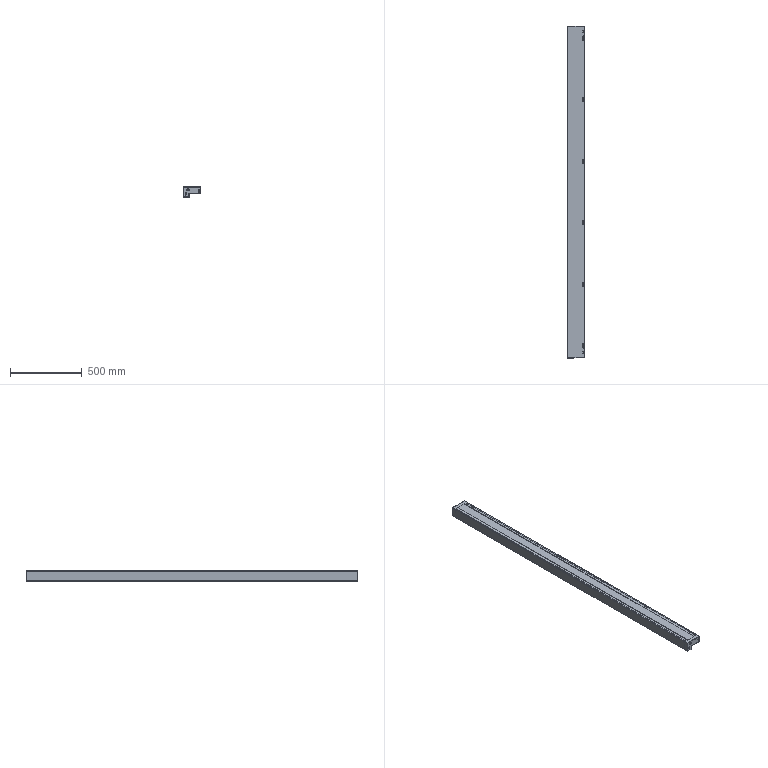Part | 5 solids | 342 faces | box 120 x 2316 x 70 mm | volume 1328964 mm3 | plane 212 | cylinder 130 | commonest cylinder face diameters 6 x28 6.2 x28 9 x18 11 x10 3.4 x9 4 x8